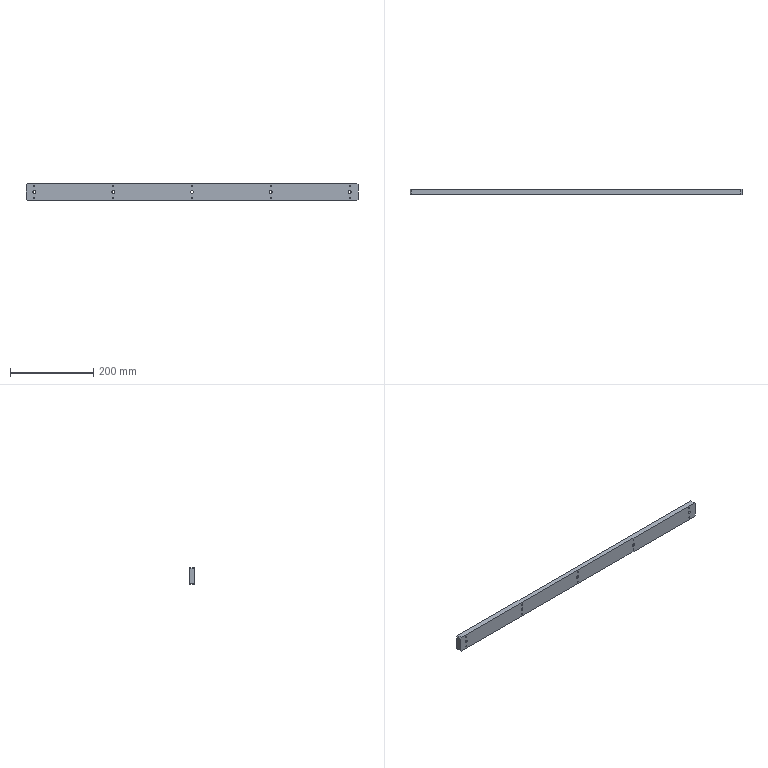Part | STEP file | DAOLIECHAO-BAN_1-2 | 1 solid | 55 faces | box 800 x 12 x 40 mm | volume 378698 mm3 | cylinder 40 | plane 15 | commonest cylinder face diameters 3.3 x20 6.6 x10 11 x10